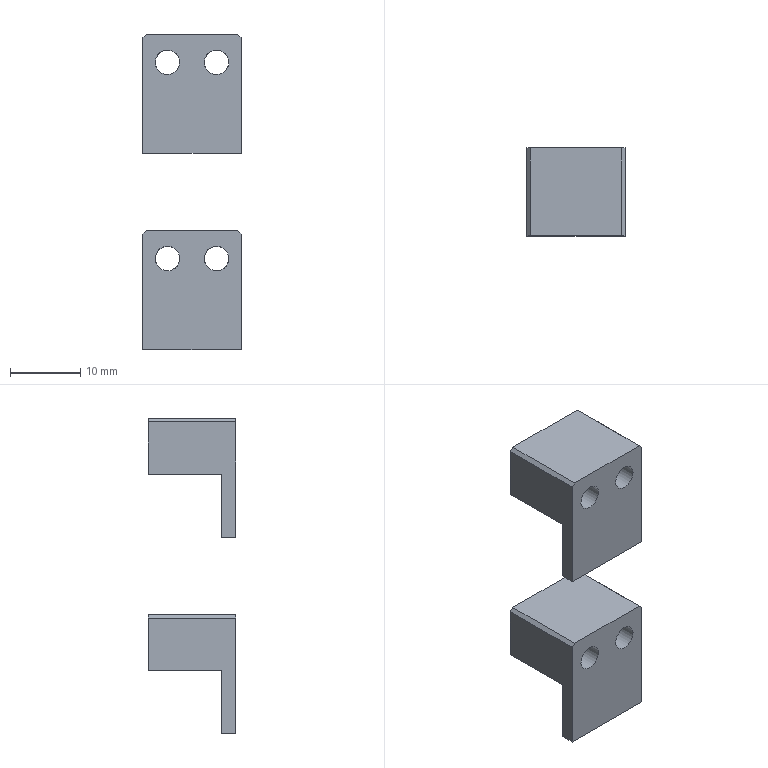Part | NX | 2 solids | 24 faces | box 14 x 12.5 x 45 mm | volume 2817 mm3 | plane 20 | cylinder 4 | commonest cylinder face diameters 3.5 x4
STEP:
#1=CARTESIAN_POINT('',(71.444,336.443,-249.3));
#2=VERTEX_POINT('',#1);
#3=CARTESIAN_POINT('',(70.944,336.443,-249.8));
#4=VERTEX_POINT('',#3);
#5=CARTESIAN_POINT('',(65.694,336.443,-255.05));
#6=DIRECTION('',(-0.7071,0.,-0.7071));
#7=VECTOR('',#6,1000.);
#8=LINE('',#5,#7);
#9=EDGE_CURVE('',#2,#4,#8,.T.);
#10=ORIENTED_EDGE('',*,*,#9,.F.);
#11=CARTESIAN_POINT('',(71.444,348.943,-249.3));
#12=VERTEX_POINT('',#11);
#13=CARTESIAN_POINT('',(71.444,336.443,-249.3));
#14=DIRECTION('',(0.,-1.,0.));
#15=VECTOR('',#14,1000.);
#16=LINE('',#13,#15);
#17=EDGE_CURVE('',#12,#2,#16,.T.);
#18=ORIENTED_EDGE('',*,*,#17,.F.);
#19=CARTESIAN_POINT('',(70.944,348.943,-249.8));
#20=VERTEX_POINT('',#19);
#21=CARTESIAN_POINT('',(63.219,348.943,-257.525));
#22=DIRECTION('',(0.7071,0.,0.7071));
#23=VECTOR('',#22,1000.);
#24=LINE('',#21,#23);
#25=EDGE_CURVE('',#20,#12,#24,.T.);
#26=ORIENTED_EDGE('',*,*,#25,.F.);
#27=CARTESIAN_POINT('',(70.944,348.943,-249.8));
#28=DIRECTION('',(0.,1.,0.));
#29=VECTOR('',#28,1000.);
#30=LINE('',#27,#29);
#31=EDGE_CURVE('',#4,#20,#30,.T.);
#32=ORIENTED_EDGE('',*,*,#31,.F.);
#33=EDGE_LOOP('',(#10,#18,#26,#32));
#34=FACE_BOUND('',#33,.T.);
#35=CARTESIAN_POINT('',(70.944,336.943,-249.8));
#36=DIRECTION('',(-0.7071,0.,0.7071));
#37=DIRECTION('',(0.,-1.,0.));
#38=AXIS2_PLACEMENT_3D('',#35,#36,#37);
#39=PLANE('',#38);
#40=ADVANCED_FACE('',(#34),#39,.T.);
#41=CARTESIAN_POINT('',(84.444,348.943,-249.3));
#42=VERTEX_POINT('',#41);
#43=CARTESIAN_POINT('',(84.944,348.943,-249.8));
#44=VERTEX_POINT('',#43);
#45=CARTESIAN_POINT('',(47.369,348.943,-212.225));
#46=DIRECTION('',(0.7071,0.,-0.7071));
#47=VECTOR('',#46,1000.);
#48=LINE('',#45,#47);
#49=EDGE_CURVE('',#42,#44,#48,.T.);
#50=ORIENTED_EDGE('',*,*,#49,.F.);
#51=CARTESIAN_POINT('',(84.444,336.443,-249.3));
#52=VERTEX_POINT('',#51);
#53=CARTESIAN_POINT('',(84.444,348.943,-249.3));
#54=DIRECTION('',(0.,1.,0.));
#55=VECTOR('',#54,1000.);
#56=LINE('',#53,#55);
#57=EDGE_CURVE('',#52,#42,#56,.T.);
#58=ORIENTED_EDGE('',*,*,#57,.F.);
#59=CARTESIAN_POINT('',(84.944,336.443,-249.8));
#60=VERTEX_POINT('',#59);
#61=CARTESIAN_POINT('',(85.044,336.443,-249.9));
#62=DIRECTION('',(-0.7071,0.,0.7071));
#63=VECTOR('',#62,1000.);
#64=LINE('',#61,#63);
#65=EDGE_CURVE('',#60,#52,#64,.T.);
#66=ORIENTED_EDGE('',*,*,#65,.F.);
#67=CARTESIAN_POINT('',(84.944,336.443,-249.8));
#68=DIRECTION('',(0.,-1.,0.));
#69=VECTOR('',#68,1000.);
#70=LINE('',#67,#69);
#71=EDGE_CURVE('',#44,#60,#70,.T.);
#72=ORIENTED_EDGE('',*,*,#71,.F.);
#73=EDGE_LOOP('',(#50,#58,#66,#72));
#74=FACE_BOUND('',#73,.T.);
#75=CARTESIAN_POINT('',(84.944,336.943,-249.8));
#76=DIRECTION('',(0.7071,0.,0.7071));
#77=DIRECTION('',(0.,1.,0.));
#78=AXIS2_PLACEMENT_3D('',#75,#76,#77);
#79=PLANE('',#78);
#80=ADVANCED_FACE('',(#74),#79,.T.);
#81=CARTESIAN_POINT('',(76.194,348.943,-253.3));
#82=VERTEX_POINT('',#81);
#83=CARTESIAN_POINT('',(74.444,348.943,-253.3));
#84=DIRECTION('',(0.,-1.,0.));
#85=DIRECTION('',(1.,0.,0.));
#86=AXIS2_PLACEMENT_3D('',#83,#84,#85);
#87=CIRCLE('',#86,1.75);
#88=EDGE_CURVE('',#82,#82,#87,.T.);
#89=ORIENTED_EDGE('',*,*,#88,.F.);
#90=EDGE_LOOP('',(#89));
#91=FACE_BOUND('',#90,.T.);
#92=CARTESIAN_POINT('',(74.444,336.443,-255.05));
#93=VERTEX_POINT('',#92);
#94=CARTESIAN_POINT('',(74.444,336.443,-253.3));
#95=DIRECTION('',(0.,-1.,0.));
#96=DIRECTION('',(0.,0.,-1.));
#97=AXIS2_PLACEMENT_3D('',#94,#95,#96);
#98=CIRCLE('',#97,1.75);
#99=EDGE_CURVE('',#93,#93,#98,.T.);
#100=ORIENTED_EDGE('',*,*,#99,.T.);
#101=EDGE_LOOP('',(#100));
#102=FACE_BOUND('',#101,.T.);
#103=CARTESIAN_POINT('',(74.444,348.943,-253.3));
#104=DIRECTION('',(0.,-1.,0.));
#105=DIRECTION('',(1.,0.,0.));
#106=AXIS2_PLACEMENT_3D('',#103,#104,#105);
#107=CYLINDRICAL_SURFACE('',#106,1.75);
#108=ADVANCED_FACE('',(#91,#102),#107,.F.);
#109=CARTESIAN_POINT('',(83.194,348.943,-253.3));
#110=VERTEX_POINT('',#109);
#111=CARTESIAN_POINT('',(81.444,348.943,-253.3));
#112=DIRECTION('',(0.,-1.,0.));
#113=DIRECTION('',(1.,0.,0.));
#114=AXIS2_PLACEMENT_3D('',#111,#112,#113);
#115=CIRCLE('',#114,1.75);
#116=EDGE_CURVE('',#110,#110,#115,.T.);
#117=ORIENTED_EDGE('',*,*,#116,.F.);
#118=EDGE_LOOP('',(#117));
#119=FACE_BOUND('',#118,.T.);
#120=CARTESIAN_POINT('',(81.444,336.443,-255.05));
#121=VERTEX_POINT('',#120);
#122=CARTESIAN_POINT('',(81.444,336.443,-253.3));
#123=DIRECTION('',(0.,-1.,0.));
#124=DIRECTION('',(0.,0.,-1.));
#125=AXIS2_PLACEMENT_3D('',#122,#123,#124);
#126=CIRCLE('',#125,1.75);
#127=EDGE_CURVE('',#121,#121,#126,.T.);
#128=ORIENTED_EDGE('',*,*,#127,.T.);
#129=EDGE_LOOP('',(#128));
#130=FACE_BOUND('',#129,.T.);
#131=CARTESIAN_POINT('',(81.444,348.943,-253.3));
#132=DIRECTION('',(0.,-1.,0.));
#133=DIRECTION('',(1.,0.,0.));
#134=AXIS2_PLACEMENT_3D('',#131,#132,#133);
#135=CYLINDRICAL_SURFACE('',#134,1.75);
#136=ADVANCED_FACE('',(#119,#130),#135,.F.);
#137=CARTESIAN_POINT('',(77.973,336.443,-249.3));
#138=DIRECTION('',(-1.,0.,0.));
#139=VECTOR('',#138,1000.);
#140=LINE('',#137,#139);
#141=EDGE_CURVE('',#52,#2,#140,.T.);
#142=ORIENTED_EDGE('',*,*,#141,.F.);
#143=ORIENTED_EDGE('',*,*,#57,.T.);
#144=CARTESIAN_POINT('',(32.644,348.943,-249.3));
#145=DIRECTION('',(-1.,0.,0.));
#146=VECTOR('',#145,1000.);
#147=LINE('',#144,#146);
#148=EDGE_CURVE('',#42,#12,#147,.T.);
#149=ORIENTED_EDGE('',*,*,#148,.T.);
#150=ORIENTED_EDGE('',*,*,#17,.T.);
#151=EDGE_LOOP('',(#142,#143,#149,#150));
#152=FACE_BOUND('',#151,.T.);
#153=CARTESIAN_POINT('',(77.973,336.443,-249.3));
#154=DIRECTION('',(0.,0.,-1.));
#155=DIRECTION('',(-1.,0.,0.));
#156=AXIS2_PLACEMENT_3D('',#153,#154,#155);
#157=PLANE('',#156);
#158=ADVANCED_FACE('',(#152),#157,.F.);
#159=CARTESIAN_POINT('',(70.944,338.443,-257.3));
#160=VERTEX_POINT('',#159);
#161=CARTESIAN_POINT('',(70.944,338.443,-266.3));
#162=VERTEX_POINT('',#161);
#163=CARTESIAN_POINT('',(70.944,338.443,-262.15));
#164=DIRECTION('',(0.,0.,-1.));
#165=VECTOR('',#164,1000.);
#166=LINE('',#163,#165);
#167=EDGE_CURVE('',#160,#162,#166,.T.);
#168=ORIENTED_EDGE('',*,*,#167,.F.);
#169=CARTESIAN_POINT('',(84.944,338.443,-257.3));
#170=VERTEX_POINT('',#169);
#171=CARTESIAN_POINT('',(72.794,338.443,-257.3));
#172=DIRECTION('',(1.,0.,0.));
#173=VECTOR('',#172,1000.);
#174=LINE('',#171,#173);
#175=EDGE_CURVE('',#160,#170,#174,.T.);
#176=ORIENTED_EDGE('',*,*,#175,.T.);
#177=CARTESIAN_POINT('',(84.944,338.443,-266.3));
#178=VERTEX_POINT('',#177);
#179=CARTESIAN_POINT('',(84.944,338.443,-262.15));
#180=DIRECTION('',(0.,0.,1.));
#181=VECTOR('',#180,1000.);
#182=LINE('',#179,#181);
#183=EDGE_CURVE('',#178,#170,#182,.T.);
#184=ORIENTED_EDGE('',*,*,#183,.F.);
#185=CARTESIAN_POINT('',(72.794,338.443,-266.3));
#186=DIRECTION('',(1.,0.,0.));
#187=VECTOR('',#186,1000.);
#188=LINE('',#185,#187);
#189=EDGE_CURVE('',#162,#178,#188,.T.);
#190=ORIENTED_EDGE('',*,*,#189,.F.);
#191=EDGE_LOOP('',(#168,#176,#184,#190));
#192=FACE_BOUND('',#191,.T.);
#193=CARTESIAN_POINT('',(72.794,338.443,-262.15));
#194=DIRECTION('',(0.,1.,0.));
#195=DIRECTION('',(-1.,0.,0.));
#196=AXIS2_PLACEMENT_3D('',#193,#194,#195);
#197=PLANE('',#196);
#198=ADVANCED_FACE('',(#192),#197,.T.);
#199=CARTESIAN_POINT('',(84.944,336.443,-266.3));
#200=VERTEX_POINT('',#199);
#201=CARTESIAN_POINT('',(84.944,336.943,-266.3));
#202=DIRECTION('',(0.,-1.,0.));
#203=VECTOR('',#202,1000.);
#204=LINE('',#201,#203);
#205=EDGE_CURVE('',#178,#200,#204,.T.);
#206=ORIENTED_EDGE('',*,*,#205,.T.);
#207=CARTESIAN_POINT('',(70.944,336.443,-266.3));
#208=VERTEX_POINT('',#207);
#209=CARTESIAN_POINT('',(72.794,336.443,-266.3));
#210=DIRECTION('',(-1.,0.,0.));
#211=VECTOR('',#210,1000.);
#212=LINE('',#209,#211);
#213=EDGE_CURVE('',#200,#208,#212,.T.);
#214=ORIENTED_EDGE('',*,*,#213,.T.);
#215=CARTESIAN_POINT('',(70.944,336.943,-266.3));
#216=DIRECTION('',(0.,-1.,0.));
#217=VECTOR('',#216,1000.);
#218=LINE('',#215,#217);
#219=EDGE_CURVE('',#162,#208,#218,.T.);
#220=ORIENTED_EDGE('',*,*,#219,.F.);
#221=ORIENTED_EDGE('',*,*,#189,.T.);
#222=EDGE_LOOP('',(#206,#214,#220,#221));
#223=FACE_BOUND('',#222,.T.);
#224=CARTESIAN_POINT('',(72.794,336.943,-266.3));
#225=DIRECTION('',(0.,0.,-1.));
#226=DIRECTION('',(0.,1.,0.));
#227=AXIS2_PLACEMENT_3D('',#224,#225,#226);
#228=PLANE('',#227);
#229=ADVANCED_FACE('',(#223),#228,.T.);
#230=CARTESIAN_POINT('',(84.944,348.943,-257.3));
#231=VERTEX_POINT('',#230);
#232=CARTESIAN_POINT('',(84.944,348.943,-262.15));
#233=DIRECTION('',(0.,0.,1.));
#234=VECTOR('',#233,1000.);
#235=LINE('',#232,#234);
#236=EDGE_CURVE('',#231,#44,#235,.T.);
#237=ORIENTED_EDGE('',*,*,#236,.T.);
#238=ORIENTED_EDGE('',*,*,#71,.T.);
#239=CARTESIAN_POINT('',(84.944,336.443,-262.15));
#240=DIRECTION('',(0.,0.,-1.));
#241=VECTOR('',#240,1000.);
#242=LINE('',#239,#241);
#243=EDGE_CURVE('',#60,#200,#242,.T.);
#244=ORIENTED_EDGE('',*,*,#243,.T.);
#245=ORIENTED_EDGE('',*,*,#205,.F.);
#246=ORIENTED_EDGE('',*,*,#183,.T.);
#247=CARTESIAN_POINT('',(84.944,336.943,-257.3));
#248=DIRECTION('',(0.,-1.,0.));
#249=VECTOR('',#248,1000.);
#250=LINE('',#247,#249);
#251=EDGE_CURVE('',#231,#170,#250,.T.);
#252=ORIENTED_EDGE('',*,*,#251,.F.);
#253=EDGE_LOOP('',(#237,#238,#244,#245,#246,#252));
#254=FACE_BOUND('',#253,.T.);
#255=CARTESIAN_POINT('',(84.944,336.943,-262.15));
#256=DIRECTION('',(1.,0.,0.));
#257=DIRECTION('',(0.,1.,0.));
#258=AXIS2_PLACEMENT_3D('',#255,#256,#257);
#259=PLANE('',#258);
#260=ADVANCED_FACE('',(#254),#259,.T.);
#261=ORIENTED_EDGE('',*,*,#148,.F.);
#262=ORIENTED_EDGE('',*,*,#49,.T.);
#263=ORIENTED_EDGE('',*,*,#236,.F.);
#264=CARTESIAN_POINT('',(70.944,348.943,-257.3));
#265=VERTEX_POINT('',#264);
#266=CARTESIAN_POINT('',(72.794,348.943,-257.3));
#267=DIRECTION('',(-1.,0.,0.));
#268=VECTOR('',#267,1000.);
#269=LINE('',#266,#268);
#270=EDGE_CURVE('',#231,#265,#269,.T.);
#271=ORIENTED_EDGE('',*,*,#270,.T.);
#272=CARTESIAN_POINT('',(70.944,348.943,-262.15));
#273=DIRECTION('',(0.,0.,-1.));
#274=VECTOR('',#273,1000.);
#275=LINE('',#272,#274);
#276=EDGE_CURVE('',#20,#265,#275,.T.);
#277=ORIENTED_EDGE('',*,*,#276,.F.);
#278=ORIENTED_EDGE('',*,*,#25,.T.);
#279=EDGE_LOOP('',(#261,#262,#263,#271,#277,#278));
#280=FACE_BOUND('',#279,.T.);
#281=ORIENTED_EDGE('',*,*,#116,.T.);
#282=EDGE_LOOP('',(#281));
#283=FACE_BOUND('',#282,.T.);
#284=ORIENTED_EDGE('',*,*,#88,.T.);
#285=EDGE_LOOP('',(#284));
#286=FACE_BOUND('',#285,.T.);
#287=CARTESIAN_POINT('',(32.644,348.943,-226.95));
#288=DIRECTION('',(0.,1.,0.));
#289=DIRECTION('',(0.,0.,-1.));
#290=AXIS2_PLACEMENT_3D('',#287,#288,#289);
#291=PLANE('',#290);
#292=ADVANCED_FACE('',(#280,#283,#286),#291,.T.);
#293=CARTESIAN_POINT('',(70.944,336.443,-262.15));
#294=DIRECTION('',(0.,0.,1.));
#295=VECTOR('',#294,1000.);
#296=LINE('',#293,#295);
#297=EDGE_CURVE('',#208,#4,#296,.T.);
#298=ORIENTED_EDGE('',*,*,#297,.T.);
#299=ORIENTED_EDGE('',*,*,#31,.T.);
#300=ORIENTED_EDGE('',*,*,#276,.T.);
#301=CARTESIAN_POINT('',(70.944,336.943,-257.3));
#302=DIRECTION('',(0.,1.,0.));
#303=VECTOR('',#302,1000.);
#304=LINE('',#301,#303);
#305=EDGE_CURVE('',#160,#265,#304,.T.);
#306=ORIENTED_EDGE('',*,*,#305,.F.);
#307=ORIENTED_EDGE('',*,*,#167,.T.);
#308=ORIENTED_EDGE('',*,*,#219,.T.);
#309=EDGE_LOOP('',(#298,#299,#300,#306,#307,#308));
#310=FACE_BOUND('',#309,.T.);
#311=CARTESIAN_POINT('',(70.944,336.943,-262.15));
#312=DIRECTION('',(-1.,0.,0.));
#313=DIRECTION('',(0.,-1.,0.));
#314=AXIS2_PLACEMENT_3D('',#311,#312,#313);
#315=PLANE('',#314);
#316=ADVANCED_FACE('',(#310),#315,.T.);
#317=ORIENTED_EDGE('',*,*,#243,.F.);
#318=ORIENTED_EDGE('',*,*,#65,.T.);
#319=ORIENTED_EDGE('',*,*,#141,.T.);
#320=ORIENTED_EDGE('',*,*,#9,.T.);
#321=ORIENTED_EDGE('',*,*,#297,.F.);
#322=ORIENTED_EDGE('',*,*,#213,.F.);
#323=EDGE_LOOP('',(#317,#318,#319,#320,#321,#322));
#324=FACE_BOUND('',#323,.T.);
#325=ORIENTED_EDGE('',*,*,#127,.F.);
#326=EDGE_LOOP('',(#325));
#327=FACE_BOUND('',#326,.T.);
#328=ORIENTED_EDGE('',*,*,#99,.F.);
#329=EDGE_LOOP('',(#328));
#330=FACE_BOUND('',#329,.T.);
#331=CARTESIAN_POINT('',(72.794,336.443,-262.15));
#332=DIRECTION('',(0.,-1.,0.));
#333=DIRECTION('',(1.,0.,0.));
#334=AXIS2_PLACEMENT_3D('',#331,#332,#333);
#335=PLANE('',#334);
#336=ADVANCED_FACE('',(#324,#327,#330),#335,.T.);
#337=ORIENTED_EDGE('',*,*,#175,.F.);
#338=ORIENTED_EDGE('',*,*,#305,.T.);
#339=ORIENTED_EDGE('',*,*,#270,.F.);
#340=ORIENTED_EDGE('',*,*,#251,.T.);
#341=EDGE_LOOP('',(#337,#338,#339,#340));
#342=FACE_BOUND('',#341,.T.);
#343=CARTESIAN_POINT('',(72.794,339.081,-257.3));
#344=DIRECTION('',(0.,0.,1.));
#345=DIRECTION('',(0.,-1.,0.));
#346=AXIS2_PLACEMENT_3D('',#343,#344,#345);
#347=PLANE('',#346);
#348=ADVANCED_FACE('',(#342),#347,.F.);
#349=CLOSED_SHELL('',(#40,#80,#108,#136,#158,#198,#229,#260,#292,#316,#336,#348));
#350=MANIFOLD_SOLID_BREP('',#349);
#351=CARTESIAN_POINT('',(71.444,336.443,-221.3));
#352=VERTEX_POINT('',#351);
#353=CARTESIAN_POINT('',(70.944,336.443,-221.8));
#354=VERTEX_POINT('',#353);
#355=CARTESIAN_POINT('',(65.694,336.443,-227.05));
#356=DIRECTION('',(-0.7071,0.,-0.7071));
#357=VECTOR('',#356,1000.);
#358=LINE('',#355,#357);
#359=EDGE_CURVE('',#352,#354,#358,.T.);
#360=ORIENTED_EDGE('',*,*,#359,.F.);
#361=CARTESIAN_POINT('',(71.444,348.943,-221.3));
#362=VERTEX_POINT('',#361);
#363=CARTESIAN_POINT('',(71.444,336.443,-221.3));
#364=DIRECTION('',(0.,-1.,0.));
#365=VECTOR('',#364,1000.);
#366=LINE('',#363,#365);
#367=EDGE_CURVE('',#362,#352,#366,.T.);
#368=ORIENTED_EDGE('',*,*,#367,.F.);
#369=CARTESIAN_POINT('',(70.944,348.943,-221.8));
#370=VERTEX_POINT('',#369);
#371=CARTESIAN_POINT('',(63.219,348.943,-229.525));
#372=DIRECTION('',(0.7071,0.,0.7071));
#373=VECTOR('',#372,1000.);
#374=LINE('',#371,#373);
#375=EDGE_CURVE('',#370,#362,#374,.T.);
#376=ORIENTED_EDGE('',*,*,#375,.F.);
#377=CARTESIAN_POINT('',(70.944,348.943,-221.8));
#378=DIRECTION('',(0.,1.,0.));
#379=VECTOR('',#378,1000.);
#380=LINE('',#377,#379);
#381=EDGE_CURVE('',#354,#370,#380,.T.);
#382=ORIENTED_EDGE('',*,*,#381,.F.);
#383=EDGE_LOOP('',(#360,#368,#376,#382));
#384=FACE_BOUND('',#383,.T.);
#385=CARTESIAN_POINT('',(70.944,336.943,-221.8));
#386=DIRECTION('',(-0.7071,0.,0.7071));
#387=DIRECTION('',(0.,-1.,0.));
#388=AXIS2_PLACEMENT_3D('',#385,#386,#387);
#389=PLANE('',#388);
#390=ADVANCED_FACE('',(#384),#389,.T.);
#391=CARTESIAN_POINT('',(84.444,348.943,-221.3));
#392=VERTEX_POINT('',#391);
#393=CARTESIAN_POINT('',(84.944,348.943,-221.8));
#394=VERTEX_POINT('',#393);
#395=CARTESIAN_POINT('',(47.369,348.943,-184.225));
#396=DIRECTION('',(0.7071,0.,-0.7071));
#397=VECTOR('',#396,1000.);
#398=LINE('',#395,#397);
#399=EDGE_CURVE('',#392,#394,#398,.T.);
#400=ORIENTED_EDGE('',*,*,#399,.F.);
#401=CARTESIAN_POINT('',(84.444,336.443,-221.3));
#402=VERTEX_POINT('',#401);
#403=CARTESIAN_POINT('',(84.444,348.943,-221.3));
#404=DIRECTION('',(0.,1.,0.));
#405=VECTOR('',#404,1000.);
#406=LINE('',#403,#405);
#407=EDGE_CURVE('',#402,#392,#406,.T.);
#408=ORIENTED_EDGE('',*,*,#407,.F.);
#409=CARTESIAN_POINT('',(84.944,336.443,-221.8));
#410=VERTEX_POINT('',#409);
#411=CARTESIAN_POINT('',(85.044,336.443,-221.9));
#412=DIRECTION('',(-0.7071,0.,0.7071));
#413=VECTOR('',#412,1000.);
#414=LINE('',#411,#413);
#415=EDGE_CURVE('',#410,#402,#414,.T.);
#416=ORIENTED_EDGE('',*,*,#415,.F.);
#417=CARTESIAN_POINT('',(84.944,336.443,-221.8));
#418=DIRECTION('',(0.,-1.,0.));
#419=VECTOR('',#418,1000.);
#420=LINE('',#417,#419);
#421=EDGE_CURVE('',#394,#410,#420,.T.);
#422=ORIENTED_EDGE('',*,*,#421,.F.);
#423=EDGE_LOOP('',(#400,#408,#416,#422));
#424=FACE_BOUND('',#423,.T.);
#425=CARTESIAN_POINT('',(84.944,336.943,-221.8));
#426=DIRECTION('',(0.7071,0.,0.7071));
#427=DIRECTION('',(0.,1.,0.));
#428=AXIS2_PLACEMENT_3D('',#425,#426,#427);
#429=PLANE('',#428);
#430=ADVANCED_FACE('',(#424),#429,.T.);
#431=CARTESIAN_POINT('',(76.194,348.943,-225.3));
#432=VERTEX_POINT('',#431);
#433=CARTESIAN_POINT('',(74.444,348.943,-225.3));
#434=DIRECTION('',(0.,-1.,0.));
#435=DIRECTION('',(1.,0.,0.));
#436=AXIS2_PLACEMENT_3D('',#433,#434,#435);
#437=CIRCLE('',#436,1.75);
#438=EDGE_CURVE('',#432,#432,#437,.T.);
#439=ORIENTED_EDGE('',*,*,#438,.F.);
#440=EDGE_LOOP('',(#439));
#441=FACE_BOUND('',#440,.T.);
#442=CARTESIAN_POINT('',(74.444,336.443,-227.05));
#443=VERTEX_POINT('',#442);
#444=CARTESIAN_POINT('',(74.444,336.443,-225.3));
#445=DIRECTION('',(0.,-1.,0.));
#446=DIRECTION('',(0.,0.,-1.));
#447=AXIS2_PLACEMENT_3D('',#444,#445,#446);
#448=CIRCLE('',#447,1.75);
#449=EDGE_CURVE('',#443,#443,#448,.T.);
#450=ORIENTED_EDGE('',*,*,#449,.T.);
#451=EDGE_LOOP('',(#450));
#452=FACE_BOUND('',#451,.T.);
#453=CARTESIAN_POINT('',(74.444,348.943,-225.3));
#454=DIRECTION('',(0.,-1.,0.));
#455=DIRECTION('',(1.,0.,0.));
#456=AXIS2_PLACEMENT_3D('',#453,#454,#455);
#457=CYLINDRICAL_SURFACE('',#456,1.75);
#458=ADVANCED_FACE('',(#441,#452),#457,.F.);
#459=CARTESIAN_POINT('',(83.194,348.943,-225.3));
#460=VERTEX_POINT('',#459);
#461=CARTESIAN_POINT('',(81.444,348.943,-225.3));
#462=DIRECTION('',(0.,-1.,0.));
#463=DIRECTION('',(1.,0.,0.));
#464=AXIS2_PLACEMENT_3D('',#461,#462,#463);
#465=CIRCLE('',#464,1.75);
#466=EDGE_CURVE('',#460,#460,#465,.T.);
#467=ORIENTED_EDGE('',*,*,#466,.F.);
#468=EDGE_LOOP('',(#467));
#469=FACE_BOUND('',#468,.T.);
#470=CARTESIAN_POINT('',(81.444,336.443,-227.05));
#471=VERTEX_POINT('',#470);
#472=CARTESIAN_POINT('',(81.444,336.443,-225.3));
#473=DIRECTION('',(0.,-1.,0.));
#474=DIRECTION('',(0.,0.,-1.));
#475=AXIS2_PLACEMENT_3D('',#472,#473,#474);
#476=CIRCLE('',#475,1.75);
#477=EDGE_CURVE('',#471,#471,#476,.T.);
#478=ORIENTED_EDGE('',*,*,#477,.T.);
#479=EDGE_LOOP('',(#478));
#480=FACE_BOUND('',#479,.T.);
#481=CARTESIAN_POINT('',(81.444,348.943,-225.3));
#482=DIRECTION('',(0.,-1.,0.));
#483=DIRECTION('',(1.,0.,0.));
#484=AXIS2_PLACEMENT_3D('',#481,#482,#483);
#485=CYLINDRICAL_SURFACE('',#484,1.75);
#486=ADVANCED_FACE('',(#469,#480),#485,.F.);
#487=CARTESIAN_POINT('',(77.973,336.443,-221.3));
#488=DIRECTION('',(-1.,0.,0.));
#489=VECTOR('',#488,1000.);
#490=LINE('',#487,#489);
#491=EDGE_CURVE('',#402,#352,#490,.T.);
#492=ORIENTED_EDGE('',*,*,#491,.F.);
#493=ORIENTED_EDGE('',*,*,#407,.T.);
#494=CARTESIAN_POINT('',(32.644,348.943,-221.3));
#495=DIRECTION('',(-1.,0.,0.));
#496=VECTOR('',#495,1000.);
#497=LINE('',#494,#496);
#498=EDGE_CURVE('',#392,#362,#497,.T.);
#499=ORIENTED_EDGE('',*,*,#498,.T.);
#500=ORIENTED_EDGE('',*,*,#367,.T.);
#501=EDGE_LOOP('',(#492,#493,#499,#500));
#502=FACE_BOUND('',#501,.T.);
#503=CARTESIAN_POINT('',(77.973,336.443,-221.3));
#504=DIRECTION('',(0.,0.,-1.));
#505=DIRECTION('',(-1.,0.,0.));
#506=AXIS2_PLACEMENT_3D('',#503,#504,#505);
#507=PLANE('',#506);
#508=ADVANCED_FACE('',(#502),#507,.F.);
#509=CARTESIAN_POINT('',(70.944,338.443,-229.3));
#510=VERTEX_POINT('',#509);
#511=CARTESIAN_POINT('',(70.944,338.443,-238.3));
#512=VERTEX_POINT('',#511);
#513=CARTESIAN_POINT('',(70.944,338.443,-234.15));
#514=DIRECTION('',(0.,0.,-1.));
#515=VECTOR('',#514,1000.);
#516=LINE('',#513,#515);
#517=EDGE_CURVE('',#510,#512,#516,.T.);
#518=ORIENTED_EDGE('',*,*,#517,.F.);
#519=CARTESIAN_POINT('',(84.944,338.443,-229.3));
#520=VERTEX_POINT('',#519);
#521=CARTESIAN_POINT('',(72.794,338.443,-229.3));
#522=DIRECTION('',(1.,0.,0.));
#523=VECTOR('',#522,1000.);
#524=LINE('',#521,#523);
#525=EDGE_CURVE('',#510,#520,#524,.T.);
#526=ORIENTED_EDGE('',*,*,#525,.T.);
#527=CARTESIAN_POINT('',(84.944,338.443,-238.3));
#528=VERTEX_POINT('',#527);
#529=CARTESIAN_POINT('',(84.944,338.443,-234.15));
#530=DIRECTION('',(0.,0.,1.));
#531=VECTOR('',#530,1000.);
#532=LINE('',#529,#531);
#533=EDGE_CURVE('',#528,#520,#532,.T.);
#534=ORIENTED_EDGE('',*,*,#533,.F.);
#535=CARTESIAN_POINT('',(72.794,338.443,-238.3));
#536=DIRECTION('',(1.,0.,0.));
#537=VECTOR('',#536,1000.);
#538=LINE('',#535,#537);
#539=EDGE_CURVE('',#512,#528,#538,.T.);
#540=ORIENTED_EDGE('',*,*,#539,.F.);
#541=EDGE_LOOP('',(#518,#526,#534,#540));
#542=FACE_BOUND('',#541,.T.);
#543=CARTESIAN_POINT('',(72.794,338.443,-234.15));
#544=DIRECTION('',(0.,1.,0.));
#545=DIRECTION('',(-1.,0.,0.));
#546=AXIS2_PLACEMENT_3D('',#543,#544,#545);
#547=PLANE('',#546);
#548=ADVANCED_FACE('',(#542),#547,.T.);
#549=CARTESIAN_POINT('',(84.944,336.443,-238.3));
#550=VERTEX_POINT('',#549);
#551=CARTESIAN_POINT('',(84.944,336.943,-238.3));
#552=DIRECTION('',(0.,-1.,0.));
#553=VECTOR('',#552,1000.);
#554=LINE('',#551,#553);
#555=EDGE_CURVE('',#528,#550,#554,.T.);
#556=ORIENTED_EDGE('',*,*,#555,.T.);
#557=CARTESIAN_POINT('',(70.944,336.443,-238.3));
#558=VERTEX_POINT('',#557);
#559=CARTESIAN_POINT('',(72.794,336.443,-238.3));
#560=DIRECTION('',(-1.,0.,0.));
#561=VECTOR('',#560,1000.);
#562=LINE('',#559,#561);
#563=EDGE_CURVE('',#550,#558,#562,.T.);
#564=ORIENTED_EDGE('',*,*,#563,.T.);
#565=CARTESIAN_POINT('',(70.944,336.943,-238.3));
#566=DIRECTION('',(0.,-1.,0.));
#567=VECTOR('',#566,1000.);
#568=LINE('',#565,#567);
#569=EDGE_CURVE('',#512,#558,#568,.T.);
#570=ORIENTED_EDGE('',*,*,#569,.F.);
#571=ORIENTED_EDGE('',*,*,#539,.T.);
#572=EDGE_LOOP('',(#556,#564,#570,#571));
#573=FACE_BOUND('',#572,.T.);
#574=CARTESIAN_POINT('',(72.794,336.943,-238.3));
#575=DIRECTION('',(0.,0.,-1.));
#576=DIRECTION('',(0.,1.,0.));
#577=AXIS2_PLACEMENT_3D('',#574,#575,#576);
#578=PLANE('',#577);
#579=ADVANCED_FACE('',(#573),#578,.T.);
#580=CARTESIAN_POINT('',(84.944,348.943,-229.3));
#581=VERTEX_POINT('',#580);
#582=CARTESIAN_POINT('',(84.944,348.943,-234.15));
#583=DIRECTION('',(0.,0.,1.));
#584=VECTOR('',#583,1000.);
#585=LINE('',#582,#584);
#586=EDGE_CURVE('',#581,#394,#585,.T.);
#587=ORIENTED_EDGE('',*,*,#586,.T.);
#588=ORIENTED_EDGE('',*,*,#421,.T.);
#589=CARTESIAN_POINT('',(84.944,336.443,-234.15));
#590=DIRECTION('',(0.,0.,-1.));
#591=VECTOR('',#590,1000.);
#592=LINE('',#589,#591);
#593=EDGE_CURVE('',#410,#550,#592,.T.);
#594=ORIENTED_EDGE('',*,*,#593,.T.);
#595=ORIENTED_EDGE('',*,*,#555,.F.);
#596=ORIENTED_EDGE('',*,*,#533,.T.);
#597=CARTESIAN_POINT('',(84.944,336.943,-229.3));
#598=DIRECTION('',(0.,-1.,0.));
#599=VECTOR('',#598,1000.);
#600=LINE('',#597,#599);
#601=EDGE_CURVE('',#581,#520,#600,.T.);
#602=ORIENTED_EDGE('',*,*,#601,.F.);
#603=EDGE_LOOP('',(#587,#588,#594,#595,#596,#602));
#604=FACE_BOUND('',#603,.T.);
#605=CARTESIAN_POINT('',(84.944,336.943,-234.15));
#606=DIRECTION('',(1.,0.,0.));
#607=DIRECTION('',(0.,1.,0.));
#608=AXIS2_PLACEMENT_3D('',#605,#606,#607);
#609=PLANE('',#608);
#610=ADVANCED_FACE('',(#604),#609,.T.);
#611=ORIENTED_EDGE('',*,*,#498,.F.);
#612=ORIENTED_EDGE('',*,*,#399,.T.);
#613=ORIENTED_EDGE('',*,*,#586,.F.);
#614=CARTESIAN_POINT('',(70.944,348.943,-229.3));
#615=VERTEX_POINT('',#614);
#616=CARTESIAN_POINT('',(72.794,348.943,-229.3));
#617=DIRECTION('',(-1.,0.,0.));
#618=VECTOR('',#617,1000.);
#619=LINE('',#616,#618);
#620=EDGE_CURVE('',#581,#615,#619,.T.);
#621=ORIENTED_EDGE('',*,*,#620,.T.);
#622=CARTESIAN_POINT('',(70.944,348.943,-234.15));
#623=DIRECTION('',(0.,0.,-1.));
#624=VECTOR('',#623,1000.);
#625=LINE('',#622,#624);
#626=EDGE_CURVE('',#370,#615,#625,.T.);
#627=ORIENTED_EDGE('',*,*,#626,.F.);
#628=ORIENTED_EDGE('',*,*,#375,.T.);
#629=EDGE_LOOP('',(#611,#612,#613,#621,#627,#628));
#630=FACE_BOUND('',#629,.T.);
#631=ORIENTED_EDGE('',*,*,#466,.T.);
#632=EDGE_LOOP('',(#631));
#633=FACE_BOUND('',#632,.T.);
#634=ORIENTED_EDGE('',*,*,#438,.T.);
#635=EDGE_LOOP('',(#634));
#636=FACE_BOUND('',#635,.T.);
#637=CARTESIAN_POINT('',(32.644,348.943,-198.95));
#638=DIRECTION('',(0.,1.,0.));
#639=DIRECTION('',(0.,0.,-1.));
#640=AXIS2_PLACEMENT_3D('',#637,#638,#639);
#641=PLANE('',#640);
#642=ADVANCED_FACE('',(#630,#633,#636),#641,.T.);
#643=CARTESIAN_POINT('',(70.944,336.443,-234.15));
#644=DIRECTION('',(0.,0.,1.));
#645=VECTOR('',#644,1000.);
#646=LINE('',#643,#645);
#647=EDGE_CURVE('',#558,#354,#646,.T.);
#648=ORIENTED_EDGE('',*,*,#647,.T.);
#649=ORIENTED_EDGE('',*,*,#381,.T.);
#650=ORIENTED_EDGE('',*,*,#626,.T.);
#651=CARTESIAN_POINT('',(70.944,336.943,-229.3));
#652=DIRECTION('',(0.,1.,0.));
#653=VECTOR('',#652,1000.);
#654=LINE('',#651,#653);
#655=EDGE_CURVE('',#510,#615,#654,.T.);
#656=ORIENTED_EDGE('',*,*,#655,.F.);
#657=ORIENTED_EDGE('',*,*,#517,.T.);
#658=ORIENTED_EDGE('',*,*,#569,.T.);
#659=EDGE_LOOP('',(#648,#649,#650,#656,#657,#658));
#660=FACE_BOUND('',#659,.T.);
#661=CARTESIAN_POINT('',(70.944,336.943,-234.15));
#662=DIRECTION('',(-1.,0.,0.));
#663=DIRECTION('',(0.,-1.,0.));
#664=AXIS2_PLACEMENT_3D('',#661,#662,#663);
#665=PLANE('',#664);
#666=ADVANCED_FACE('',(#660),#665,.T.);
#667=ORIENTED_EDGE('',*,*,#593,.F.);
#668=ORIENTED_EDGE('',*,*,#415,.T.);
#669=ORIENTED_EDGE('',*,*,#491,.T.);
#670=ORIENTED_EDGE('',*,*,#359,.T.);
#671=ORIENTED_EDGE('',*,*,#647,.F.);
#672=ORIENTED_EDGE('',*,*,#563,.F.);
#673=EDGE_LOOP('',(#667,#668,#669,#670,#671,#672));
#674=FACE_BOUND('',#673,.T.);
#675=ORIENTED_EDGE('',*,*,#477,.F.);
#676=EDGE_LOOP('',(#675));
#677=FACE_BOUND('',#676,.T.);
#678=ORIENTED_EDGE('',*,*,#449,.F.);
#679=EDGE_LOOP('',(#678));
#680=FACE_BOUND('',#679,.T.);
#681=CARTESIAN_POINT('',(72.794,336.443,-234.15));
#682=DIRECTION('',(0.,-1.,0.));
#683=DIRECTION('',(1.,0.,0.));
#684=AXIS2_PLACEMENT_3D('',#681,#682,#683);
#685=PLANE('',#684);
#686=ADVANCED_FACE('',(#674,#677,#680),#685,.T.);
#687=ORIENTED_EDGE('',*,*,#525,.F.);
#688=ORIENTED_EDGE('',*,*,#655,.T.);
#689=ORIENTED_EDGE('',*,*,#620,.F.);
#690=ORIENTED_EDGE('',*,*,#601,.T.);
#691=EDGE_LOOP('',(#687,#688,#689,#690));
#692=FACE_BOUND('',#691,.T.);
#693=CARTESIAN_POINT('',(72.794,339.081,-229.3));
#694=DIRECTION('',(0.,0.,1.));
#695=DIRECTION('',(0.,-1.,0.));
#696=AXIS2_PLACEMENT_3D('',#693,#694,#695);
#697=PLANE('',#696);
#698=ADVANCED_FACE('',(#692),#697,.F.);
#699=CLOSED_SHELL('',(#390,#430,#458,#486,#508,#548,#579,#610,#642,#666,#686,#698));
#700=MANIFOLD_SOLID_BREP('',#699);
#701=(LENGTH_UNIT()NAMED_UNIT(*)SI_UNIT(.MILLI.,.METRE.));
#702=UNCERTAINTY_MEASURE_WITH_UNIT(LENGTH_MEASURE(0.00001),#701,'','');
#703=(NAMED_UNIT(*)PLANE_ANGLE_UNIT()SI_UNIT($,.RADIAN.));
#704=(NAMED_UNIT(*)SI_UNIT($,.STERADIAN.)SOLID_ANGLE_UNIT());
#705=(GEOMETRIC_REPRESENTATION_CONTEXT(3)GLOBAL_UNCERTAINTY_ASSIGNED_CONTEXT((#702))GLOBAL_UNIT_ASSIGNED_CONTEXT((#701,#703,#704))REPRESENTATION_CONTEXT('',''));
#706=ADVANCED_BREP_SHAPE_REPRESENTATION('',(#350,#700),#705);